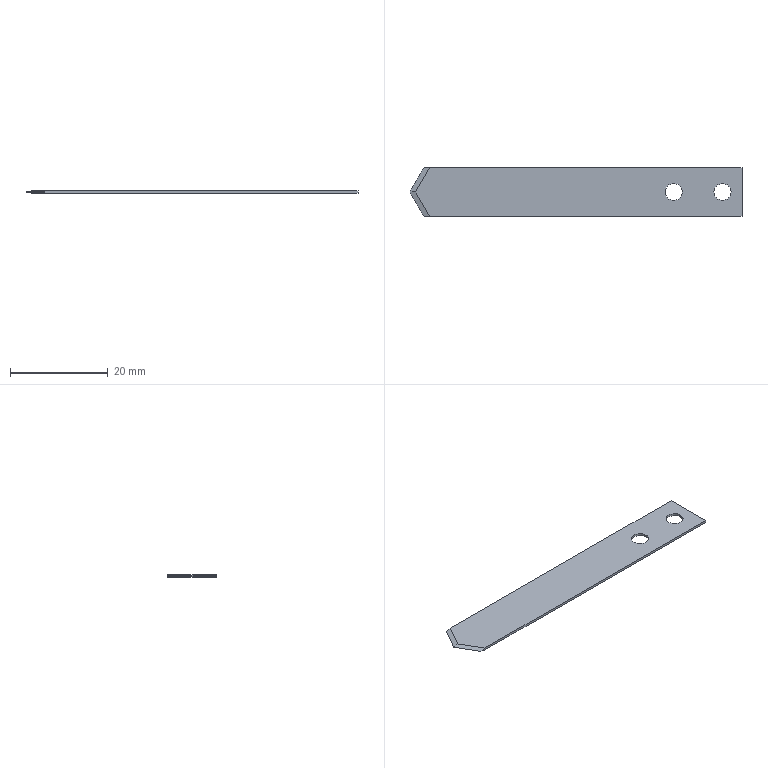Part | NX | features BREP 1 | 1 solid | 15 faces | box 68 x 10 x 0.5 mm | volume 320.283 mm3 | plane 11 | cylinder 4 | commonest cylinder face diameters 3.5 x4
STEP:
#1=CARTESIAN_POINT('',(28.25,0.,-0.25));
#2=VERTEX_POINT('',#1);
#3=CARTESIAN_POINT('',(31.75,0.,-0.25));
#4=VERTEX_POINT('',#3);
#5=CARTESIAN_POINT('',(30.,0.,-0.25));
#6=DIRECTION('',(0.,0.,1.));
#7=DIRECTION('',(1.,0.,0.));
#8=AXIS2_PLACEMENT_3D('',#5,#6,#7);
#9=CIRCLE('',#8,1.75);
#10=EDGE_CURVE('',#2,#4,#9,.T.);
#11=ORIENTED_EDGE('',*,*,#10,.F.);
#12=CARTESIAN_POINT('',(28.25,0.,0.25));
#13=VERTEX_POINT('',#12);
#14=CARTESIAN_POINT('',(28.25,0.,-0.25));
#15=DIRECTION('',(0.,0.,1.));
#16=VECTOR('',#15,1000.);
#17=LINE('',#14,#16);
#18=EDGE_CURVE('',#2,#13,#17,.T.);
#19=ORIENTED_EDGE('',*,*,#18,.T.);
#20=CARTESIAN_POINT('',(31.75,0.,0.25));
#21=VERTEX_POINT('',#20);
#22=CARTESIAN_POINT('',(30.,0.,0.25));
#23=DIRECTION('',(0.,0.,-1.));
#24=DIRECTION('',(-1.,0.,0.));
#25=AXIS2_PLACEMENT_3D('',#22,#23,#24);
#26=CIRCLE('',#25,1.75);
#27=EDGE_CURVE('',#21,#13,#26,.T.);
#28=ORIENTED_EDGE('',*,*,#27,.F.);
#29=CARTESIAN_POINT('',(31.75,0.,-0.25));
#30=DIRECTION('',(0.,0.,1.));
#31=VECTOR('',#30,1000.);
#32=LINE('',#29,#31);
#33=EDGE_CURVE('',#4,#21,#32,.T.);
#34=ORIENTED_EDGE('',*,*,#33,.F.);
#35=EDGE_LOOP('',(#11,#19,#28,#34));
#36=FACE_BOUND('',#35,.T.);
#37=CARTESIAN_POINT('',(30.,0.,-0.25));
#38=DIRECTION('',(0.,0.,1.));
#39=DIRECTION('',(-1.,0.,0.));
#40=AXIS2_PLACEMENT_3D('',#37,#38,#39);
#41=CYLINDRICAL_SURFACE('',#40,1.75);
#42=ADVANCED_FACE('',(#36),#41,.F.);
#43=CARTESIAN_POINT('',(18.25,0.,-0.25));
#44=VERTEX_POINT('',#43);
#45=CARTESIAN_POINT('',(21.75,0.,-0.25));
#46=VERTEX_POINT('',#45);
#47=CARTESIAN_POINT('',(20.,0.,-0.25));
#48=DIRECTION('',(0.,0.,1.));
#49=DIRECTION('',(1.,0.,0.));
#50=AXIS2_PLACEMENT_3D('',#47,#48,#49);
#51=CIRCLE('',#50,1.75);
#52=EDGE_CURVE('',#44,#46,#51,.T.);
#53=ORIENTED_EDGE('',*,*,#52,.F.);
#54=CARTESIAN_POINT('',(18.25,0.,0.25));
#55=VERTEX_POINT('',#54);
#56=CARTESIAN_POINT('',(18.25,0.,-0.25));
#57=DIRECTION('',(0.,0.,1.));
#58=VECTOR('',#57,1000.);
#59=LINE('',#56,#58);
#60=EDGE_CURVE('',#44,#55,#59,.T.);
#61=ORIENTED_EDGE('',*,*,#60,.T.);
#62=CARTESIAN_POINT('',(21.75,0.,0.25));
#63=VERTEX_POINT('',#62);
#64=CARTESIAN_POINT('',(20.,0.,0.25));
#65=DIRECTION('',(0.,0.,-1.));
#66=DIRECTION('',(-1.,0.,0.));
#67=AXIS2_PLACEMENT_3D('',#64,#65,#66);
#68=CIRCLE('',#67,1.75);
#69=EDGE_CURVE('',#63,#55,#68,.T.);
#70=ORIENTED_EDGE('',*,*,#69,.F.);
#71=CARTESIAN_POINT('',(21.75,0.,-0.25));
#72=DIRECTION('',(0.,0.,1.));
#73=VECTOR('',#72,1000.);
#74=LINE('',#71,#73);
#75=EDGE_CURVE('',#46,#63,#74,.T.);
#76=ORIENTED_EDGE('',*,*,#75,.F.);
#77=EDGE_LOOP('',(#53,#61,#70,#76));
#78=FACE_BOUND('',#77,.T.);
#79=CARTESIAN_POINT('',(20.,0.,-0.25));
#80=DIRECTION('',(0.,0.,1.));
#81=DIRECTION('',(-1.,0.,0.));
#82=AXIS2_PLACEMENT_3D('',#79,#80,#81);
#83=CYLINDRICAL_SURFACE('',#82,1.75);
#84=ADVANCED_FACE('',(#78),#83,.F.);
#85=ORIENTED_EDGE('',*,*,#27,.T.);
#86=CARTESIAN_POINT('',(30.,0.,0.25));
#87=DIRECTION('',(0.,0.,-1.));
#88=DIRECTION('',(-1.,0.,0.));
#89=AXIS2_PLACEMENT_3D('',#86,#87,#88);
#90=CIRCLE('',#89,1.75);
#91=EDGE_CURVE('',#13,#21,#90,.T.);
#92=ORIENTED_EDGE('',*,*,#91,.T.);
#93=EDGE_LOOP('',(#85,#92));
#94=FACE_BOUND('',#93,.T.);
#95=ORIENTED_EDGE('',*,*,#69,.T.);
#96=CARTESIAN_POINT('',(20.,0.,0.25));
#97=DIRECTION('',(0.,0.,-1.));
#98=DIRECTION('',(-1.,0.,0.));
#99=AXIS2_PLACEMENT_3D('',#96,#97,#98);
#100=CIRCLE('',#99,1.75);
#101=EDGE_CURVE('',#55,#63,#100,.T.);
#102=ORIENTED_EDGE('',*,*,#101,.T.);
#103=EDGE_LOOP('',(#95,#102));
#104=FACE_BOUND('',#103,.T.);
#105=CARTESIAN_POINT('',(-29.959,5.,0.25));
#106=VERTEX_POINT('',#105);
#107=CARTESIAN_POINT('',(34.,5.,0.25));
#108=VERTEX_POINT('',#107);
#109=CARTESIAN_POINT('',(-34.,5.,0.25));
#110=DIRECTION('',(1.,0.,0.));
#111=VECTOR('',#110,1000.);
#112=LINE('',#109,#111);
#113=EDGE_CURVE('',#106,#108,#112,.T.);
#114=ORIENTED_EDGE('',*,*,#113,.F.);
#115=CARTESIAN_POINT('',(-32.845,0.,0.25));
#116=VERTEX_POINT('',#115);
#117=CARTESIAN_POINT('',(-33.134,-0.5,0.25));
#118=DIRECTION('',(-0.5,-0.866,0.));
#119=VECTOR('',#118,1000.);
#120=LINE('',#117,#119);
#121=EDGE_CURVE('',#106,#116,#120,.T.);
#122=ORIENTED_EDGE('',*,*,#121,.T.);
#123=CARTESIAN_POINT('',(-29.959,-5.,0.25));
#124=VERTEX_POINT('',#123);
#125=CARTESIAN_POINT('',(-30.247,-4.5,0.25));
#126=DIRECTION('',(0.5,-0.866,0.));
#127=VECTOR('',#126,1000.);
#128=LINE('',#125,#127);
#129=EDGE_CURVE('',#116,#124,#128,.T.);
#130=ORIENTED_EDGE('',*,*,#129,.T.);
#131=CARTESIAN_POINT('',(34.,-5.,0.25));
#132=VERTEX_POINT('',#131);
#133=CARTESIAN_POINT('',(-34.,-5.,0.25));
#134=DIRECTION('',(1.,0.,0.));
#135=VECTOR('',#134,1000.);
#136=LINE('',#133,#135);
#137=EDGE_CURVE('',#124,#132,#136,.T.);
#138=ORIENTED_EDGE('',*,*,#137,.T.);
#139=CARTESIAN_POINT('',(34.,5.,0.25));
#140=DIRECTION('',(0.,-1.,0.));
#141=VECTOR('',#140,1000.);
#142=LINE('',#139,#141);
#143=EDGE_CURVE('',#108,#132,#142,.T.);
#144=ORIENTED_EDGE('',*,*,#143,.F.);
#145=EDGE_LOOP('',(#114,#122,#130,#138,#144));
#146=FACE_BOUND('',#145,.T.);
#147=CARTESIAN_POINT('',(0.,0.,0.25));
#148=DIRECTION('',(0.,0.,-1.));
#149=DIRECTION('',(1.,0.,0.));
#150=AXIS2_PLACEMENT_3D('',#147,#148,#149);
#151=PLANE('',#150);
#152=ADVANCED_FACE('',(#94,#104,#146),#151,.F.);
#153=CARTESIAN_POINT('',(30.,0.,-0.25));
#154=DIRECTION('',(0.,0.,1.));
#155=DIRECTION('',(1.,0.,0.));
#156=AXIS2_PLACEMENT_3D('',#153,#154,#155);
#157=CIRCLE('',#156,1.75);
#158=EDGE_CURVE('',#4,#2,#157,.T.);
#159=ORIENTED_EDGE('',*,*,#158,.T.);
#160=ORIENTED_EDGE('',*,*,#10,.T.);
#161=EDGE_LOOP('',(#159,#160));
#162=FACE_BOUND('',#161,.T.);
#163=CARTESIAN_POINT('',(20.,0.,-0.25));
#164=DIRECTION('',(0.,0.,1.));
#165=DIRECTION('',(1.,0.,0.));
#166=AXIS2_PLACEMENT_3D('',#163,#164,#165);
#167=CIRCLE('',#166,1.75);
#168=EDGE_CURVE('',#46,#44,#167,.T.);
#169=ORIENTED_EDGE('',*,*,#168,.T.);
#170=ORIENTED_EDGE('',*,*,#52,.T.);
#171=EDGE_LOOP('',(#169,#170));
#172=FACE_BOUND('',#171,.T.);
#173=CARTESIAN_POINT('',(-29.959,-5.,-0.25));
#174=VERTEX_POINT('',#173);
#175=CARTESIAN_POINT('',(-32.845,0.,-0.25));
#176=VERTEX_POINT('',#175);
#177=CARTESIAN_POINT('',(-24.634,-14.222,-0.25));
#178=DIRECTION('',(-0.5,0.866,0.));
#179=VECTOR('',#178,1000.);
#180=LINE('',#177,#179);
#181=EDGE_CURVE('',#174,#176,#180,.T.);
#182=ORIENTED_EDGE('',*,*,#181,.T.);
#183=CARTESIAN_POINT('',(-29.959,5.,-0.25));
#184=VERTEX_POINT('',#183);
#185=CARTESIAN_POINT('',(-24.634,14.222,-0.25));
#186=DIRECTION('',(0.5,0.866,0.));
#187=VECTOR('',#186,1000.);
#188=LINE('',#185,#187);
#189=EDGE_CURVE('',#176,#184,#188,.T.);
#190=ORIENTED_EDGE('',*,*,#189,.T.);
#191=CARTESIAN_POINT('',(34.,5.,-0.25));
#192=VERTEX_POINT('',#191);
#193=CARTESIAN_POINT('',(-34.,5.,-0.25));
#194=DIRECTION('',(1.,0.,0.));
#195=VECTOR('',#194,1000.);
#196=LINE('',#193,#195);
#197=EDGE_CURVE('',#184,#192,#196,.T.);
#198=ORIENTED_EDGE('',*,*,#197,.T.);
#199=CARTESIAN_POINT('',(34.,-5.,-0.25));
#200=VERTEX_POINT('',#199);
#201=CARTESIAN_POINT('',(34.,5.,-0.25));
#202=DIRECTION('',(0.,-1.,0.));
#203=VECTOR('',#202,1000.);
#204=LINE('',#201,#203);
#205=EDGE_CURVE('',#192,#200,#204,.T.);
#206=ORIENTED_EDGE('',*,*,#205,.T.);
#207=CARTESIAN_POINT('',(-34.,-5.,-0.25));
#208=DIRECTION('',(1.,0.,0.));
#209=VECTOR('',#208,1000.);
#210=LINE('',#207,#209);
#211=EDGE_CURVE('',#174,#200,#210,.T.);
#212=ORIENTED_EDGE('',*,*,#211,.F.);
#213=EDGE_LOOP('',(#182,#190,#198,#206,#212));
#214=FACE_BOUND('',#213,.T.);
#215=CARTESIAN_POINT('',(0.,0.,-0.25));
#216=DIRECTION('',(0.,0.,-1.));
#217=DIRECTION('',(1.,0.,0.));
#218=AXIS2_PLACEMENT_3D('',#215,#216,#217);
#219=PLANE('',#218);
#220=ADVANCED_FACE('',(#162,#172,#214),#219,.T.);
#221=ORIENTED_EDGE('',*,*,#137,.F.);
#222=CARTESIAN_POINT('',(-31.113,-5.,0.000672));
#223=VERTEX_POINT('',#222);
#224=CARTESIAN_POINT('',(-25.75,-5.,1.159));
#225=DIRECTION('',(-0.9775,0.,-0.2111));
#226=VECTOR('',#225,1000.);
#227=LINE('',#224,#226);
#228=EDGE_CURVE('',#124,#223,#227,.T.);
#229=ORIENTED_EDGE('',*,*,#228,.T.);
#230=CARTESIAN_POINT('',(-31.113,-5.,-0.000672));
#231=VERTEX_POINT('',#230);
#232=CARTESIAN_POINT('',(-31.113,-5.,-0.25));
#233=DIRECTION('',(0.,0.,1.));
#234=VECTOR('',#233,1000.);
#235=LINE('',#232,#234);
#236=EDGE_CURVE('',#231,#223,#235,.T.);
#237=ORIENTED_EDGE('',*,*,#236,.F.);
#238=CARTESIAN_POINT('',(-25.75,-5.,-1.159));
#239=DIRECTION('',(0.9775,0.,-0.2111));
#240=VECTOR('',#239,1000.);
#241=LINE('',#238,#240);
#242=EDGE_CURVE('',#231,#174,#241,.T.);
#243=ORIENTED_EDGE('',*,*,#242,.T.);
#244=ORIENTED_EDGE('',*,*,#211,.T.);
#245=CARTESIAN_POINT('',(34.,-5.,0.25));
#246=DIRECTION('',(0.,0.,-1.));
#247=VECTOR('',#246,1000.);
#248=LINE('',#245,#247);
#249=EDGE_CURVE('',#132,#200,#248,.T.);
#250=ORIENTED_EDGE('',*,*,#249,.F.);
#251=EDGE_LOOP('',(#221,#229,#237,#243,#244,#250));
#252=FACE_BOUND('',#251,.T.);
#253=CARTESIAN_POINT('',(-34.,-5.,0.25));
#254=DIRECTION('',(0.,1.,0.));
#255=DIRECTION('',(0.,0.,-1.));
#256=AXIS2_PLACEMENT_3D('',#253,#254,#255);
#257=PLANE('',#256);
#258=ADVANCED_FACE('',(#252),#257,.F.);
#259=CARTESIAN_POINT('',(-31.113,5.,-0.000672));
#260=VERTEX_POINT('',#259);
#261=CARTESIAN_POINT('',(-31.113,5.,0.000672));
#262=VERTEX_POINT('',#261);
#263=CARTESIAN_POINT('',(-31.113,5.,-0.25));
#264=DIRECTION('',(0.,0.,1.));
#265=VECTOR('',#264,1000.);
#266=LINE('',#263,#265);
#267=EDGE_CURVE('',#260,#262,#266,.T.);
#268=ORIENTED_EDGE('',*,*,#267,.T.);
#269=CARTESIAN_POINT('',(-33.82,5.,-0.5838));
#270=DIRECTION('',(0.9775,0.,0.2111));
#271=VECTOR('',#270,1000.);
#272=LINE('',#269,#271);
#273=EDGE_CURVE('',#262,#106,#272,.T.);
#274=ORIENTED_EDGE('',*,*,#273,.T.);
#275=ORIENTED_EDGE('',*,*,#113,.T.);
#276=CARTESIAN_POINT('',(34.,5.,0.25));
#277=DIRECTION('',(0.,0.,-1.));
#278=VECTOR('',#277,1000.);
#279=LINE('',#276,#278);
#280=EDGE_CURVE('',#108,#192,#279,.T.);
#281=ORIENTED_EDGE('',*,*,#280,.T.);
#282=ORIENTED_EDGE('',*,*,#197,.F.);
#283=CARTESIAN_POINT('',(-33.923,5.,0.606));
#284=DIRECTION('',(-0.9775,0.,0.2111));
#285=VECTOR('',#284,1000.);
#286=LINE('',#283,#285);
#287=EDGE_CURVE('',#184,#260,#286,.T.);
#288=ORIENTED_EDGE('',*,*,#287,.T.);
#289=EDGE_LOOP('',(#268,#274,#275,#281,#282,#288));
#290=FACE_BOUND('',#289,.T.);
#291=CARTESIAN_POINT('',(-34.,5.,0.25));
#292=DIRECTION('',(0.,1.,0.));
#293=DIRECTION('',(0.,0.,-1.));
#294=AXIS2_PLACEMENT_3D('',#291,#292,#293);
#295=PLANE('',#294);
#296=ADVANCED_FACE('',(#290),#295,.T.);
#297=ORIENTED_EDGE('',*,*,#205,.F.);
#298=ORIENTED_EDGE('',*,*,#280,.F.);
#299=ORIENTED_EDGE('',*,*,#143,.T.);
#300=ORIENTED_EDGE('',*,*,#249,.T.);
#301=EDGE_LOOP('',(#297,#298,#299,#300));
#302=FACE_BOUND('',#301,.T.);
#303=CARTESIAN_POINT('',(34.,5.,0.25));
#304=DIRECTION('',(1.,0.,0.));
#305=DIRECTION('',(0.,0.,1.));
#306=AXIS2_PLACEMENT_3D('',#303,#304,#305);
#307=PLANE('',#306);
#308=ADVANCED_FACE('',(#302),#307,.T.);
#309=CARTESIAN_POINT('',(-34.,0.,-0.000672));
#310=VERTEX_POINT('',#309);
#311=CARTESIAN_POINT('',(-34.,0.,0.000672));
#312=VERTEX_POINT('',#311);
#313=CARTESIAN_POINT('',(-34.,0.,-0.25));
#314=DIRECTION('',(0.,0.,1.));
#315=VECTOR('',#314,1000.);
#316=LINE('',#313,#315);
#317=EDGE_CURVE('',#310,#312,#316,.T.);
#318=ORIENTED_EDGE('',*,*,#317,.T.);
#319=CARTESIAN_POINT('',(-31.113,5.,0.000672));
#320=DIRECTION('',(0.5,0.866,0.));
#321=VECTOR('',#320,1000.);
#322=LINE('',#319,#321);
#323=EDGE_CURVE('',#312,#262,#322,.T.);
#324=ORIENTED_EDGE('',*,*,#323,.T.);
#325=ORIENTED_EDGE('',*,*,#267,.F.);
#326=CARTESIAN_POINT('',(-25.5,14.722,-0.000672));
#327=DIRECTION('',(-0.5,-0.866,0.));
#328=VECTOR('',#327,1000.);
#329=LINE('',#326,#328);
#330=EDGE_CURVE('',#260,#310,#329,.T.);
#331=ORIENTED_EDGE('',*,*,#330,.T.);
#332=EDGE_LOOP('',(#318,#324,#325,#331));
#333=FACE_BOUND('',#332,.T.);
#334=CARTESIAN_POINT('',(-25.5,14.722,-0.25));
#335=DIRECTION('',(-0.866,0.5,0.));
#336=DIRECTION('',(0.5,0.866,0.));
#337=AXIS2_PLACEMENT_3D('',#334,#335,#336);
#338=PLANE('',#337);
#339=ADVANCED_FACE('',(#333),#338,.T.);
#340=ORIENTED_EDGE('',*,*,#236,.T.);
#341=CARTESIAN_POINT('',(-34.,0.,0.000672));
#342=DIRECTION('',(-0.5,0.866,0.));
#343=VECTOR('',#342,1000.);
#344=LINE('',#341,#343);
#345=EDGE_CURVE('',#223,#312,#344,.T.);
#346=ORIENTED_EDGE('',*,*,#345,.T.);
#347=ORIENTED_EDGE('',*,*,#317,.F.);
#348=CARTESIAN_POINT('',(-25.5,-14.722,-0.000672));
#349=DIRECTION('',(0.5,-0.866,0.));
#350=VECTOR('',#349,1000.);
#351=LINE('',#348,#350);
#352=EDGE_CURVE('',#310,#231,#351,.T.);
#353=ORIENTED_EDGE('',*,*,#352,.T.);
#354=EDGE_LOOP('',(#340,#346,#347,#353));
#355=FACE_BOUND('',#354,.T.);
#356=CARTESIAN_POINT('',(-25.5,-14.722,-0.25));
#357=DIRECTION('',(-0.866,-0.5,0.));
#358=DIRECTION('',(-0.5,0.866,0.));
#359=AXIS2_PLACEMENT_3D('',#356,#357,#358);
#360=PLANE('',#359);
#361=ADVANCED_FACE('',(#355),#360,.T.);
#362=ORIENTED_EDGE('',*,*,#60,.F.);
#363=ORIENTED_EDGE('',*,*,#168,.F.);
#364=ORIENTED_EDGE('',*,*,#75,.T.);
#365=ORIENTED_EDGE('',*,*,#101,.F.);
#366=EDGE_LOOP('',(#362,#363,#364,#365));
#367=FACE_BOUND('',#366,.T.);
#368=CARTESIAN_POINT('',(20.,0.,-0.25));
#369=DIRECTION('',(0.,0.,1.));
#370=DIRECTION('',(-1.,0.,0.));
#371=AXIS2_PLACEMENT_3D('',#368,#369,#370);
#372=CYLINDRICAL_SURFACE('',#371,1.75);
#373=ADVANCED_FACE('',(#367),#372,.F.);
#374=ORIENTED_EDGE('',*,*,#18,.F.);
#375=ORIENTED_EDGE('',*,*,#158,.F.);
#376=ORIENTED_EDGE('',*,*,#33,.T.);
#377=ORIENTED_EDGE('',*,*,#91,.F.);
#378=EDGE_LOOP('',(#374,#375,#376,#377));
#379=FACE_BOUND('',#378,.T.);
#380=CARTESIAN_POINT('',(30.,0.,-0.25));
#381=DIRECTION('',(0.,0.,1.));
#382=DIRECTION('',(-1.,0.,0.));
#383=AXIS2_PLACEMENT_3D('',#380,#381,#382);
#384=CYLINDRICAL_SURFACE('',#383,1.75);
#385=ADVANCED_FACE('',(#379),#384,.F.);
#386=ORIENTED_EDGE('',*,*,#228,.F.);
#387=ORIENTED_EDGE('',*,*,#129,.F.);
#388=CARTESIAN_POINT('',(-25.879,0.,1.754));
#389=DIRECTION('',(0.9775,0.,0.2111));
#390=VECTOR('',#389,1000.);
#391=LINE('',#388,#390);
#392=EDGE_CURVE('',#312,#116,#391,.T.);
#393=ORIENTED_EDGE('',*,*,#392,.F.);
#394=ORIENTED_EDGE('',*,*,#345,.F.);
#395=EDGE_LOOP('',(#386,#387,#393,#394));
#396=FACE_BOUND('',#395,.T.);
#397=CARTESIAN_POINT('',(-25.5,-14.722,0.000672));
#398=DIRECTION('',(-0.2095,-0.121,0.9703));
#399=DIRECTION('',(-0.5,0.866,0.));
#400=AXIS2_PLACEMENT_3D('',#397,#398,#399);
#401=PLANE('',#400);
#402=ADVANCED_FACE('',(#396),#401,.T.);
#403=ORIENTED_EDGE('',*,*,#392,.T.);
#404=ORIENTED_EDGE('',*,*,#121,.F.);
#405=ORIENTED_EDGE('',*,*,#273,.F.);
#406=ORIENTED_EDGE('',*,*,#323,.F.);
#407=EDGE_LOOP('',(#403,#404,#405,#406));
#408=FACE_BOUND('',#407,.T.);
#409=CARTESIAN_POINT('',(-25.5,14.722,0.000672));
#410=DIRECTION('',(-0.2095,0.121,0.9703));
#411=DIRECTION('',(0.5,0.866,0.));
#412=AXIS2_PLACEMENT_3D('',#409,#410,#411);
#413=PLANE('',#412);
#414=ADVANCED_FACE('',(#408),#413,.T.);
#415=ORIENTED_EDGE('',*,*,#242,.F.);
#416=ORIENTED_EDGE('',*,*,#352,.F.);
#417=CARTESIAN_POINT('',(-25.879,0.,-1.754));
#418=DIRECTION('',(-0.9775,0.,0.2111));
#419=VECTOR('',#418,1000.);
#420=LINE('',#417,#419);
#421=EDGE_CURVE('',#176,#310,#420,.T.);
#422=ORIENTED_EDGE('',*,*,#421,.F.);
#423=ORIENTED_EDGE('',*,*,#181,.F.);
#424=EDGE_LOOP('',(#415,#416,#422,#423));
#425=FACE_BOUND('',#424,.T.);
#426=CARTESIAN_POINT('',(-25.5,-14.722,-0.000672));
#427=DIRECTION('',(0.2095,0.121,0.9703));
#428=DIRECTION('',(-0.5,0.866,0.));
#429=AXIS2_PLACEMENT_3D('',#426,#427,#428);
#430=PLANE('',#429);
#431=ADVANCED_FACE('',(#425),#430,.F.);
#432=ORIENTED_EDGE('',*,*,#287,.F.);
#433=ORIENTED_EDGE('',*,*,#189,.F.);
#434=ORIENTED_EDGE('',*,*,#421,.T.);
#435=ORIENTED_EDGE('',*,*,#330,.F.);
#436=EDGE_LOOP('',(#432,#433,#434,#435));
#437=FACE_BOUND('',#436,.T.);
#438=CARTESIAN_POINT('',(-25.5,14.722,-0.000672));
#439=DIRECTION('',(0.2095,-0.121,0.9703));
#440=DIRECTION('',(0.5,0.866,0.));
#441=AXIS2_PLACEMENT_3D('',#438,#439,#440);
#442=PLANE('',#441);
#443=ADVANCED_FACE('',(#437),#442,.F.);
#444=CLOSED_SHELL('',(#42,#84,#152,#220,#258,#296,#308,#339,#361,#373,#385,#402,#414,#431,#443));
#445=MANIFOLD_SOLID_BREP('',#444);
#446=(LENGTH_UNIT()NAMED_UNIT(*)SI_UNIT(.MILLI.,.METRE.));
#447=UNCERTAINTY_MEASURE_WITH_UNIT(LENGTH_MEASURE(0.00001),#446,'','');
#448=(NAMED_UNIT(*)PLANE_ANGLE_UNIT()SI_UNIT($,.RADIAN.));
#449=(NAMED_UNIT(*)SI_UNIT($,.STERADIAN.)SOLID_ANGLE_UNIT());
#450=(GEOMETRIC_REPRESENTATION_CONTEXT(3)GLOBAL_UNCERTAINTY_ASSIGNED_CONTEXT((#447))GLOBAL_UNIT_ASSIGNED_CONTEXT((#446,#448,#449))REPRESENTATION_CONTEXT('',''));
#451=ADVANCED_BREP_SHAPE_REPRESENTATION('',(#445),#450);